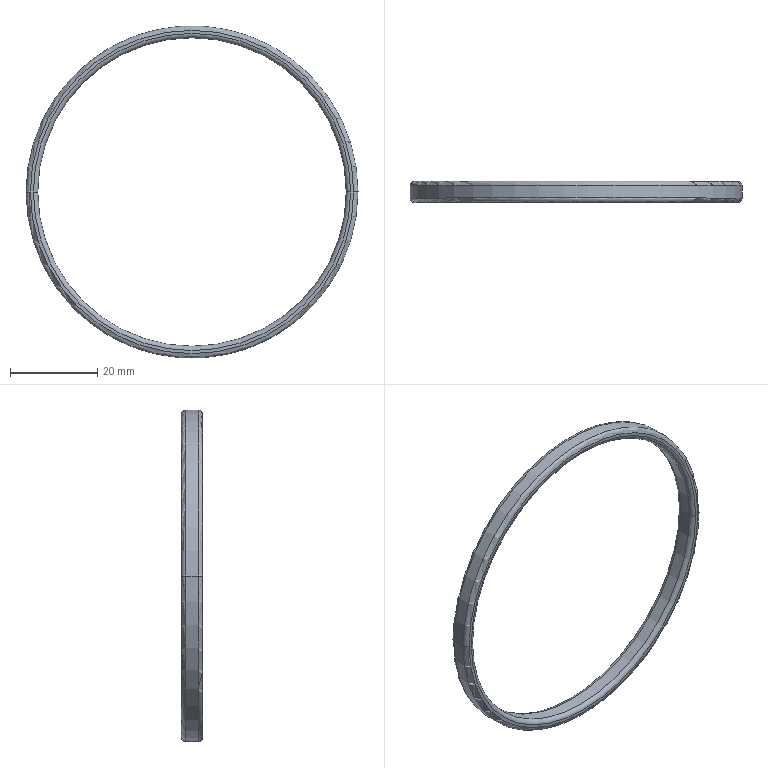Part | SolidWorks | features Revolution 1 | 1 solid | 14 faces | box 75.946 x 4.826 x 75.946 mm | volume 2793 mm3 | torus 8 | cylinder 4 | plane 2 | commonest cylinder face diameters 70.561 x2 75.946 x2
STEP:
#1=CARTESIAN_POINT('',(-36.281,10.413,0.));
#2=VERTEX_POINT('',#1);
#3=CARTESIAN_POINT('',(36.281,10.413,0.));
#4=VERTEX_POINT('',#3);
#5=CARTESIAN_POINT('',(0.,10.413,0.));
#6=DIRECTION('',(0.,1.,0.));
#7=DIRECTION('',(-1.,0.,0.));
#8=AXIS2_PLACEMENT_3D('',#5,#6,#7);
#9=CIRCLE('',#8,36.281);
#10=EDGE_CURVE('',#2,#4,#9,.T.);
#11=ORIENTED_EDGE('',*,*,#10,.T.);
#12=CARTESIAN_POINT('',(35.281,9.413,0.));
#13=VERTEX_POINT('',#12);
#14=CARTESIAN_POINT('',(36.281,9.413,0.));
#15=DIRECTION('',(0.,0.,1.));
#16=DIRECTION('',(1.,0.,0.));
#17=AXIS2_PLACEMENT_3D('',#14,#15,#16);
#18=CIRCLE('',#17,1.);
#19=EDGE_CURVE('',#4,#13,#18,.T.);
#20=ORIENTED_EDGE('',*,*,#19,.T.);
#21=CARTESIAN_POINT('',(-35.281,9.413,0.));
#22=VERTEX_POINT('',#21);
#23=CARTESIAN_POINT('',(0.,9.413,0.));
#24=DIRECTION('',(0.,1.,0.));
#25=DIRECTION('',(-1.,0.,0.));
#26=AXIS2_PLACEMENT_3D('',#23,#24,#25);
#27=CIRCLE('',#26,35.281);
#28=EDGE_CURVE('',#22,#13,#27,.T.);
#29=ORIENTED_EDGE('',*,*,#28,.F.);
#30=CARTESIAN_POINT('',(-36.281,9.413,0.));
#31=DIRECTION('',(0.,0.,-1.));
#32=DIRECTION('',(-1.,0.,0.));
#33=AXIS2_PLACEMENT_3D('',#30,#31,#32);
#34=CIRCLE('',#33,1.);
#35=EDGE_CURVE('',#2,#22,#34,.T.);
#36=ORIENTED_EDGE('',*,*,#35,.F.);
#37=EDGE_LOOP('',(#11,#20,#29,#36));
#38=FACE_OUTER_BOUND('',#37,.T.);
#39=CARTESIAN_POINT('',(0.,9.413,0.));
#40=DIRECTION('',(0.,1.,0.));
#41=DIRECTION('',(-1.,0.,0.));
#42=AXIS2_PLACEMENT_3D('',#39,#40,#41);
#43=TOROIDAL_SURFACE('',#42,36.281,1.);
#44=ADVANCED_FACE('',(#38),#43,.T.);
#45=CARTESIAN_POINT('',(35.281,6.587,0.));
#46=VERTEX_POINT('',#45);
#47=CARTESIAN_POINT('',(-35.281,6.587,0.));
#48=VERTEX_POINT('',#47);
#49=CARTESIAN_POINT('',(0.,6.587,0.));
#50=DIRECTION('',(0.,1.,0.));
#51=DIRECTION('',(-1.,0.,0.));
#52=AXIS2_PLACEMENT_3D('',#49,#50,#51);
#53=CIRCLE('',#52,35.281);
#54=EDGE_CURVE('',#46,#48,#53,.T.);
#55=ORIENTED_EDGE('',*,*,#54,.F.);
#56=CARTESIAN_POINT('',(35.281,27.,0.));
#57=DIRECTION('',(0.,1.,0.));
#58=VECTOR('',#57,1000.);
#59=LINE('',#56,#58);
#60=EDGE_CURVE('',#46,#13,#59,.T.);
#61=ORIENTED_EDGE('',*,*,#60,.T.);
#62=CARTESIAN_POINT('',(0.,9.413,0.));
#63=DIRECTION('',(0.,1.,0.));
#64=DIRECTION('',(-1.,0.,0.));
#65=AXIS2_PLACEMENT_3D('',#62,#63,#64);
#66=CIRCLE('',#65,35.281);
#67=EDGE_CURVE('',#13,#22,#66,.T.);
#68=ORIENTED_EDGE('',*,*,#67,.T.);
#69=CARTESIAN_POINT('',(-35.281,27.,0.));
#70=DIRECTION('',(0.,1.,0.));
#71=VECTOR('',#70,1000.);
#72=LINE('',#69,#71);
#73=EDGE_CURVE('',#48,#22,#72,.T.);
#74=ORIENTED_EDGE('',*,*,#73,.F.);
#75=EDGE_LOOP('',(#55,#61,#68,#74));
#76=FACE_OUTER_BOUND('',#75,.T.);
#77=CARTESIAN_POINT('',(0.,27.,0.));
#78=DIRECTION('',(0.,1.,0.));
#79=DIRECTION('',(-1.,0.,0.));
#80=AXIS2_PLACEMENT_3D('',#77,#78,#79);
#81=CYLINDRICAL_SURFACE('',#80,35.281);
#82=ADVANCED_FACE('',(#76),#81,.F.);
#83=CARTESIAN_POINT('',(0.,6.587,0.));
#84=DIRECTION('',(0.,1.,0.));
#85=DIRECTION('',(-1.,0.,0.));
#86=AXIS2_PLACEMENT_3D('',#83,#84,#85);
#87=CIRCLE('',#86,35.281);
#88=EDGE_CURVE('',#48,#46,#87,.T.);
#89=ORIENTED_EDGE('',*,*,#88,.T.);
#90=CARTESIAN_POINT('',(36.281,5.587,0.));
#91=VERTEX_POINT('',#90);
#92=CARTESIAN_POINT('',(36.281,6.587,0.));
#93=DIRECTION('',(0.,0.,1.));
#94=DIRECTION('',(1.,0.,0.));
#95=AXIS2_PLACEMENT_3D('',#92,#93,#94);
#96=CIRCLE('',#95,1.);
#97=EDGE_CURVE('',#46,#91,#96,.T.);
#98=ORIENTED_EDGE('',*,*,#97,.T.);
#99=CARTESIAN_POINT('',(-36.281,5.587,0.));
#100=VERTEX_POINT('',#99);
#101=CARTESIAN_POINT('',(0.,5.587,0.));
#102=DIRECTION('',(0.,1.,0.));
#103=DIRECTION('',(-1.,0.,0.));
#104=AXIS2_PLACEMENT_3D('',#101,#102,#103);
#105=CIRCLE('',#104,36.281);
#106=EDGE_CURVE('',#100,#91,#105,.T.);
#107=ORIENTED_EDGE('',*,*,#106,.F.);
#108=CARTESIAN_POINT('',(-36.281,6.587,0.));
#109=DIRECTION('',(0.,0.,-1.));
#110=DIRECTION('',(-1.,0.,0.));
#111=AXIS2_PLACEMENT_3D('',#108,#109,#110);
#112=CIRCLE('',#111,1.);
#113=EDGE_CURVE('',#48,#100,#112,.T.);
#114=ORIENTED_EDGE('',*,*,#113,.F.);
#115=EDGE_LOOP('',(#89,#98,#107,#114));
#116=FACE_OUTER_BOUND('',#115,.T.);
#117=CARTESIAN_POINT('',(0.,6.587,0.));
#118=DIRECTION('',(0.,1.,0.));
#119=DIRECTION('',(-1.,0.,0.));
#120=AXIS2_PLACEMENT_3D('',#117,#118,#119);
#121=TOROIDAL_SURFACE('',#120,36.281,1.);
#122=ADVANCED_FACE('',(#116),#121,.T.);
#123=CARTESIAN_POINT('',(-36.973,5.587,0.));
#124=VERTEX_POINT('',#123);
#125=CARTESIAN_POINT('',(36.973,5.587,0.));
#126=VERTEX_POINT('',#125);
#127=CARTESIAN_POINT('',(0.,5.587,0.));
#128=DIRECTION('',(0.,1.,0.));
#129=DIRECTION('',(-1.,0.,0.));
#130=AXIS2_PLACEMENT_3D('',#127,#128,#129);
#131=CIRCLE('',#130,36.973);
#132=EDGE_CURVE('',#124,#126,#131,.T.);
#133=ORIENTED_EDGE('',*,*,#132,.T.);
#134=CARTESIAN_POINT('',(37.973,6.587,0.));
#135=VERTEX_POINT('',#134);
#136=CARTESIAN_POINT('',(36.973,6.587,0.));
#137=DIRECTION('',(0.,0.,1.));
#138=DIRECTION('',(1.,0.,0.));
#139=AXIS2_PLACEMENT_3D('',#136,#137,#138);
#140=CIRCLE('',#139,1.);
#141=EDGE_CURVE('',#126,#135,#140,.T.);
#142=ORIENTED_EDGE('',*,*,#141,.T.);
#143=CARTESIAN_POINT('',(-37.973,6.587,0.));
#144=VERTEX_POINT('',#143);
#145=CARTESIAN_POINT('',(0.,6.587,0.));
#146=DIRECTION('',(0.,1.,0.));
#147=DIRECTION('',(-1.,0.,0.));
#148=AXIS2_PLACEMENT_3D('',#145,#146,#147);
#149=CIRCLE('',#148,37.973);
#150=EDGE_CURVE('',#144,#135,#149,.T.);
#151=ORIENTED_EDGE('',*,*,#150,.F.);
#152=CARTESIAN_POINT('',(-36.973,6.587,0.));
#153=DIRECTION('',(0.,0.,-1.));
#154=DIRECTION('',(-1.,0.,0.));
#155=AXIS2_PLACEMENT_3D('',#152,#153,#154);
#156=CIRCLE('',#155,1.);
#157=EDGE_CURVE('',#124,#144,#156,.T.);
#158=ORIENTED_EDGE('',*,*,#157,.F.);
#159=EDGE_LOOP('',(#133,#142,#151,#158));
#160=FACE_OUTER_BOUND('',#159,.T.);
#161=CARTESIAN_POINT('',(0.,6.587,0.));
#162=DIRECTION('',(0.,1.,0.));
#163=DIRECTION('',(-1.,0.,0.));
#164=AXIS2_PLACEMENT_3D('',#161,#162,#163);
#165=TOROIDAL_SURFACE('',#164,36.973,1.);
#166=ADVANCED_FACE('',(#160),#165,.T.);
#167=ORIENTED_EDGE('',*,*,#150,.T.);
#168=CARTESIAN_POINT('',(37.973,9.413,0.));
#169=VERTEX_POINT('',#168);
#170=CARTESIAN_POINT('',(37.973,27.,0.));
#171=DIRECTION('',(0.,1.,0.));
#172=VECTOR('',#171,1000.);
#173=LINE('',#170,#172);
#174=EDGE_CURVE('',#135,#169,#173,.T.);
#175=ORIENTED_EDGE('',*,*,#174,.T.);
#176=CARTESIAN_POINT('',(-37.973,9.413,0.));
#177=VERTEX_POINT('',#176);
#178=CARTESIAN_POINT('',(0.,9.413,0.));
#179=DIRECTION('',(0.,1.,0.));
#180=DIRECTION('',(-1.,0.,0.));
#181=AXIS2_PLACEMENT_3D('',#178,#179,#180);
#182=CIRCLE('',#181,37.973);
#183=EDGE_CURVE('',#177,#169,#182,.T.);
#184=ORIENTED_EDGE('',*,*,#183,.F.);
#185=CARTESIAN_POINT('',(-37.973,27.,0.));
#186=DIRECTION('',(0.,1.,0.));
#187=VECTOR('',#186,1000.);
#188=LINE('',#185,#187);
#189=EDGE_CURVE('',#144,#177,#188,.T.);
#190=ORIENTED_EDGE('',*,*,#189,.F.);
#191=EDGE_LOOP('',(#167,#175,#184,#190));
#192=FACE_OUTER_BOUND('',#191,.T.);
#193=CARTESIAN_POINT('',(0.,27.,0.));
#194=DIRECTION('',(0.,1.,0.));
#195=DIRECTION('',(-1.,0.,0.));
#196=AXIS2_PLACEMENT_3D('',#193,#194,#195);
#197=CYLINDRICAL_SURFACE('',#196,37.973);
#198=ADVANCED_FACE('',(#192),#197,.T.);
#199=ORIENTED_EDGE('',*,*,#183,.T.);
#200=CARTESIAN_POINT('',(36.973,10.413,0.));
#201=VERTEX_POINT('',#200);
#202=CARTESIAN_POINT('',(36.973,9.413,0.));
#203=DIRECTION('',(0.,0.,1.));
#204=DIRECTION('',(1.,0.,0.));
#205=AXIS2_PLACEMENT_3D('',#202,#203,#204);
#206=CIRCLE('',#205,1.);
#207=EDGE_CURVE('',#169,#201,#206,.T.);
#208=ORIENTED_EDGE('',*,*,#207,.T.);
#209=CARTESIAN_POINT('',(-36.973,10.413,0.));
#210=VERTEX_POINT('',#209);
#211=CARTESIAN_POINT('',(0.,10.413,0.));
#212=DIRECTION('',(0.,1.,0.));
#213=DIRECTION('',(-1.,0.,0.));
#214=AXIS2_PLACEMENT_3D('',#211,#212,#213);
#215=CIRCLE('',#214,36.973);
#216=EDGE_CURVE('',#210,#201,#215,.T.);
#217=ORIENTED_EDGE('',*,*,#216,.F.);
#218=CARTESIAN_POINT('',(-36.973,9.413,0.));
#219=DIRECTION('',(0.,0.,-1.));
#220=DIRECTION('',(-1.,0.,0.));
#221=AXIS2_PLACEMENT_3D('',#218,#219,#220);
#222=CIRCLE('',#221,1.);
#223=EDGE_CURVE('',#177,#210,#222,.T.);
#224=ORIENTED_EDGE('',*,*,#223,.F.);
#225=EDGE_LOOP('',(#199,#208,#217,#224));
#226=FACE_OUTER_BOUND('',#225,.T.);
#227=CARTESIAN_POINT('',(0.,9.413,0.));
#228=DIRECTION('',(0.,1.,0.));
#229=DIRECTION('',(-1.,0.,0.));
#230=AXIS2_PLACEMENT_3D('',#227,#228,#229);
#231=TOROIDAL_SURFACE('',#230,36.973,1.);
#232=ADVANCED_FACE('',(#226),#231,.T.);
#233=ORIENTED_EDGE('',*,*,#207,.F.);
#234=CARTESIAN_POINT('',(0.,9.413,0.));
#235=DIRECTION('',(0.,1.,0.));
#236=DIRECTION('',(-1.,0.,0.));
#237=AXIS2_PLACEMENT_3D('',#234,#235,#236);
#238=CIRCLE('',#237,37.973);
#239=EDGE_CURVE('',#169,#177,#238,.T.);
#240=ORIENTED_EDGE('',*,*,#239,.T.);
#241=ORIENTED_EDGE('',*,*,#223,.T.);
#242=CARTESIAN_POINT('',(0.,10.413,0.));
#243=DIRECTION('',(0.,1.,0.));
#244=DIRECTION('',(-1.,0.,0.));
#245=AXIS2_PLACEMENT_3D('',#242,#243,#244);
#246=CIRCLE('',#245,36.973);
#247=EDGE_CURVE('',#201,#210,#246,.T.);
#248=ORIENTED_EDGE('',*,*,#247,.F.);
#249=EDGE_LOOP('',(#233,#240,#241,#248));
#250=FACE_OUTER_BOUND('',#249,.T.);
#251=CARTESIAN_POINT('',(0.,9.413,0.));
#252=DIRECTION('',(0.,1.,0.));
#253=DIRECTION('',(-1.,0.,0.));
#254=AXIS2_PLACEMENT_3D('',#251,#252,#253);
#255=TOROIDAL_SURFACE('',#254,36.973,1.);
#256=ADVANCED_FACE('',(#250),#255,.T.);
#257=ORIENTED_EDGE('',*,*,#174,.F.);
#258=CARTESIAN_POINT('',(0.,6.587,0.));
#259=DIRECTION('',(0.,1.,0.));
#260=DIRECTION('',(-1.,0.,0.));
#261=AXIS2_PLACEMENT_3D('',#258,#259,#260);
#262=CIRCLE('',#261,37.973);
#263=EDGE_CURVE('',#135,#144,#262,.T.);
#264=ORIENTED_EDGE('',*,*,#263,.T.);
#265=ORIENTED_EDGE('',*,*,#189,.T.);
#266=ORIENTED_EDGE('',*,*,#239,.F.);
#267=EDGE_LOOP('',(#257,#264,#265,#266));
#268=FACE_OUTER_BOUND('',#267,.T.);
#269=CARTESIAN_POINT('',(0.,27.,0.));
#270=DIRECTION('',(0.,1.,0.));
#271=DIRECTION('',(-1.,0.,0.));
#272=AXIS2_PLACEMENT_3D('',#269,#270,#271);
#273=CYLINDRICAL_SURFACE('',#272,37.973);
#274=ADVANCED_FACE('',(#268),#273,.T.);
#275=ORIENTED_EDGE('',*,*,#141,.F.);
#276=CARTESIAN_POINT('',(0.,5.587,0.));
#277=DIRECTION('',(0.,1.,0.));
#278=DIRECTION('',(-1.,0.,0.));
#279=AXIS2_PLACEMENT_3D('',#276,#277,#278);
#280=CIRCLE('',#279,36.973);
#281=EDGE_CURVE('',#126,#124,#280,.T.);
#282=ORIENTED_EDGE('',*,*,#281,.T.);
#283=ORIENTED_EDGE('',*,*,#157,.T.);
#284=ORIENTED_EDGE('',*,*,#263,.F.);
#285=EDGE_LOOP('',(#275,#282,#283,#284));
#286=FACE_OUTER_BOUND('',#285,.T.);
#287=CARTESIAN_POINT('',(0.,6.587,0.));
#288=DIRECTION('',(0.,1.,0.));
#289=DIRECTION('',(-1.,0.,0.));
#290=AXIS2_PLACEMENT_3D('',#287,#288,#289);
#291=TOROIDAL_SURFACE('',#290,36.973,1.);
#292=ADVANCED_FACE('',(#286),#291,.T.);
#293=ORIENTED_EDGE('',*,*,#106,.T.);
#294=CARTESIAN_POINT('',(0.,5.587,0.));
#295=DIRECTION('',(0.,1.,0.));
#296=DIRECTION('',(-1.,0.,0.));
#297=AXIS2_PLACEMENT_3D('',#294,#295,#296);
#298=CIRCLE('',#297,36.281);
#299=EDGE_CURVE('',#91,#100,#298,.T.);
#300=ORIENTED_EDGE('',*,*,#299,.T.);
#301=EDGE_LOOP('',(#293,#300));
#302=FACE_BOUND('',#301,.T.);
#303=ORIENTED_EDGE('',*,*,#132,.F.);
#304=ORIENTED_EDGE('',*,*,#281,.F.);
#305=EDGE_LOOP('',(#303,#304));
#306=FACE_OUTER_BOUND('',#305,.T.);
#307=CARTESIAN_POINT('',(-36.281,5.587,0.));
#308=DIRECTION('',(0.,-1.,0.));
#309=DIRECTION('',(1.,0.,0.));
#310=AXIS2_PLACEMENT_3D('',#307,#308,#309);
#311=PLANE('',#310);
#312=ADVANCED_FACE('',(#302,#306),#311,.T.);
#313=ORIENTED_EDGE('',*,*,#97,.F.);
#314=ORIENTED_EDGE('',*,*,#54,.T.);
#315=ORIENTED_EDGE('',*,*,#113,.T.);
#316=ORIENTED_EDGE('',*,*,#299,.F.);
#317=EDGE_LOOP('',(#313,#314,#315,#316));
#318=FACE_OUTER_BOUND('',#317,.T.);
#319=CARTESIAN_POINT('',(0.,6.587,0.));
#320=DIRECTION('',(0.,1.,0.));
#321=DIRECTION('',(-1.,0.,0.));
#322=AXIS2_PLACEMENT_3D('',#319,#320,#321);
#323=TOROIDAL_SURFACE('',#322,36.281,1.);
#324=ADVANCED_FACE('',(#318),#323,.T.);
#325=ORIENTED_EDGE('',*,*,#60,.F.);
#326=ORIENTED_EDGE('',*,*,#88,.F.);
#327=ORIENTED_EDGE('',*,*,#73,.T.);
#328=ORIENTED_EDGE('',*,*,#28,.T.);
#329=EDGE_LOOP('',(#325,#326,#327,#328));
#330=FACE_OUTER_BOUND('',#329,.T.);
#331=CARTESIAN_POINT('',(0.,27.,0.));
#332=DIRECTION('',(0.,1.,0.));
#333=DIRECTION('',(-1.,0.,0.));
#334=AXIS2_PLACEMENT_3D('',#331,#332,#333);
#335=CYLINDRICAL_SURFACE('',#334,35.281);
#336=ADVANCED_FACE('',(#330),#335,.F.);
#337=ORIENTED_EDGE('',*,*,#19,.F.);
#338=CARTESIAN_POINT('',(0.,10.413,0.));
#339=DIRECTION('',(0.,1.,0.));
#340=DIRECTION('',(-1.,0.,0.));
#341=AXIS2_PLACEMENT_3D('',#338,#339,#340);
#342=CIRCLE('',#341,36.281);
#343=EDGE_CURVE('',#4,#2,#342,.T.);
#344=ORIENTED_EDGE('',*,*,#343,.T.);
#345=ORIENTED_EDGE('',*,*,#35,.T.);
#346=ORIENTED_EDGE('',*,*,#67,.F.);
#347=EDGE_LOOP('',(#337,#344,#345,#346));
#348=FACE_OUTER_BOUND('',#347,.T.);
#349=CARTESIAN_POINT('',(0.,9.413,0.));
#350=DIRECTION('',(0.,1.,0.));
#351=DIRECTION('',(-1.,0.,0.));
#352=AXIS2_PLACEMENT_3D('',#349,#350,#351);
#353=TOROIDAL_SURFACE('',#352,36.281,1.);
#354=ADVANCED_FACE('',(#348),#353,.T.);
#355=ORIENTED_EDGE('',*,*,#216,.T.);
#356=ORIENTED_EDGE('',*,*,#247,.T.);
#357=EDGE_LOOP('',(#355,#356));
#358=FACE_OUTER_BOUND('',#357,.T.);
#359=ORIENTED_EDGE('',*,*,#10,.F.);
#360=ORIENTED_EDGE('',*,*,#343,.F.);
#361=EDGE_LOOP('',(#359,#360));
#362=FACE_BOUND('',#361,.T.);
#363=CARTESIAN_POINT('',(-36.281,10.413,0.));
#364=DIRECTION('',(0.,1.,0.));
#365=DIRECTION('',(-1.,0.,0.));
#366=AXIS2_PLACEMENT_3D('',#363,#364,#365);
#367=PLANE('',#366);
#368=ADVANCED_FACE('',(#358,#362),#367,.T.);
#369=CLOSED_SHELL('',(#44,#82,#122,#166,#198,#232,#256,#274,#292,#312,#324,#336,#354,#368));
#370=MANIFOLD_SOLID_BREP('',#369);
#371=CARTESIAN_POINT('',(0.,0.,0.));
#372=DIRECTION('',(0.,0.,1.));
#373=DIRECTION('',(1.,0.,0.));
#374=AXIS2_PLACEMENT_3D('',#371,#372,#373);
#375=(LENGTH_UNIT()NAMED_UNIT(*)SI_UNIT(.MILLI.,.METRE.));
#376=UNCERTAINTY_MEASURE_WITH_UNIT(LENGTH_MEASURE(0.00001),#375,'','');
#377=(NAMED_UNIT(*)PLANE_ANGLE_UNIT()SI_UNIT($,.RADIAN.));
#378=(NAMED_UNIT(*)SI_UNIT($,.STERADIAN.)SOLID_ANGLE_UNIT());
#379=(GEOMETRIC_REPRESENTATION_CONTEXT(3)GLOBAL_UNCERTAINTY_ASSIGNED_CONTEXT((#376))GLOBAL_UNIT_ASSIGNED_CONTEXT((#375,#377,#378))REPRESENTATION_CONTEXT('',''));
#380=ADVANCED_BREP_SHAPE_REPRESENTATION('',(#370,#374),#379);